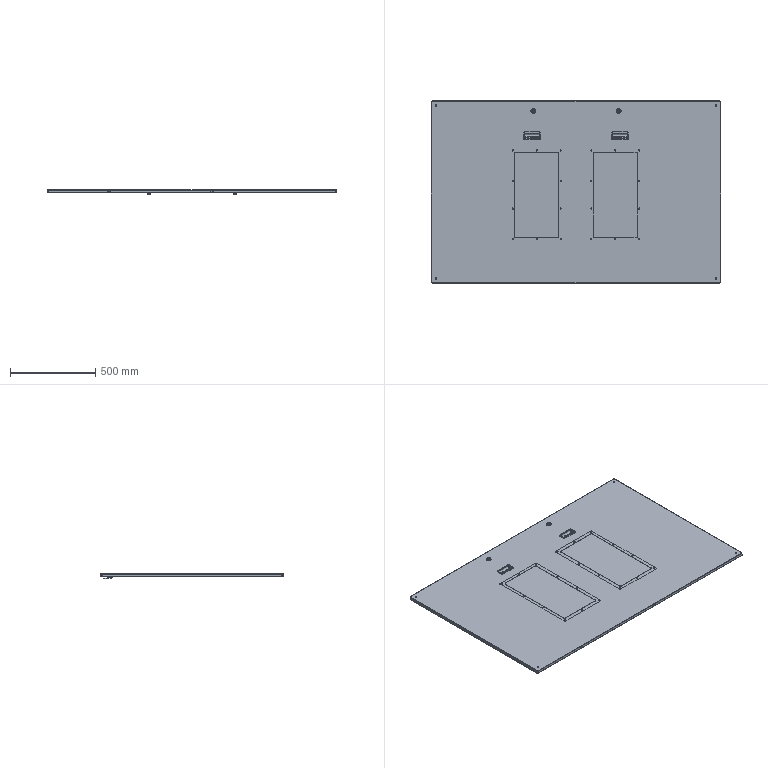Part | SolidWorks | 7 solids | 402 faces | box 1696 x 1066 x 35 mm | volume 3535734 mm3 | cylinder 190 | plane 164 | cone 40 | spline 8 | commonest cylinder face diameters 7 x80 10 x20 22 x16 9 x8 1.473 x6 2 x6